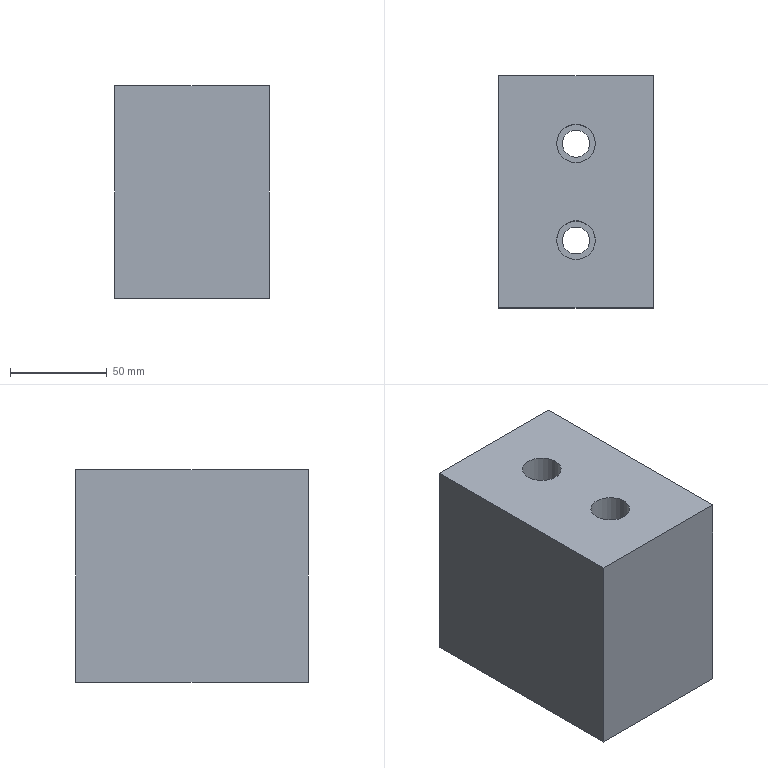Part | NX | features solid 2 | 1 solid | 12 faces | box 80 x 120 x 110 mm | volume 993294 mm3 | plane 8 | cylinder 4 | commonest cylinder face diameters 14 x2 20 x2
STEP:
#1=CARTESIAN_POINT('',(930.,850.,-30.));
#2=VERTEX_POINT('',#1);
#3=CARTESIAN_POINT('',(940.,850.,-30.));
#4=DIRECTION('',(0.,0.,-1.));
#5=DIRECTION('',(-1.,0.,0.));
#6=AXIS2_PLACEMENT_3D('',#3,#4,#5);
#7=CIRCLE('',#6,10.);
#8=EDGE_CURVE('',#2,#2,#7,.T.);
#9=ORIENTED_EDGE('',*,*,#8,.T.);
#10=EDGE_LOOP('',(#9));
#11=FACE_BOUND('',#10,.T.);
#12=CARTESIAN_POINT('',(930.,800.,-30.));
#13=VERTEX_POINT('',#12);
#14=CARTESIAN_POINT('',(940.,800.,-30.));
#15=DIRECTION('',(0.,0.,-1.));
#16=DIRECTION('',(-1.,0.,0.));
#17=AXIS2_PLACEMENT_3D('',#14,#15,#16);
#18=CIRCLE('',#17,10.);
#19=EDGE_CURVE('',#13,#13,#18,.T.);
#20=ORIENTED_EDGE('',*,*,#19,.T.);
#21=EDGE_LOOP('',(#20));
#22=FACE_BOUND('',#21,.T.);
#23=CARTESIAN_POINT('',(980.,765.,-30.));
#24=VERTEX_POINT('',#23);
#25=CARTESIAN_POINT('',(900.,765.,-30.));
#26=VERTEX_POINT('',#25);
#27=CARTESIAN_POINT('',(970.,765.,-30.));
#28=DIRECTION('',(-1.,0.,0.));
#29=VECTOR('',#28,1000.);
#30=LINE('',#27,#29);
#31=EDGE_CURVE('',#24,#26,#30,.T.);
#32=ORIENTED_EDGE('',*,*,#31,.F.);
#33=CARTESIAN_POINT('',(980.,885.,-30.));
#34=VERTEX_POINT('',#33);
#35=CARTESIAN_POINT('',(980.,880.,-30.));
#36=DIRECTION('',(0.,-1.,0.));
#37=VECTOR('',#36,1000.);
#38=LINE('',#35,#37);
#39=EDGE_CURVE('',#34,#24,#38,.T.);
#40=ORIENTED_EDGE('',*,*,#39,.F.);
#41=CARTESIAN_POINT('',(900.,885.,-30.));
#42=VERTEX_POINT('',#41);
#43=CARTESIAN_POINT('',(970.,885.,-30.));
#44=DIRECTION('',(1.,0.,0.));
#45=VECTOR('',#44,1000.);
#46=LINE('',#43,#45);
#47=EDGE_CURVE('',#34,#42,#46,.F.);
#48=ORIENTED_EDGE('',*,*,#47,.T.);
#49=CARTESIAN_POINT('',(900.,880.,-30.));
#50=DIRECTION('',(0.,-1.,0.));
#51=VECTOR('',#50,1000.);
#52=LINE('',#49,#51);
#53=EDGE_CURVE('',#42,#26,#52,.T.);
#54=ORIENTED_EDGE('',*,*,#53,.T.);
#55=EDGE_LOOP('',(#32,#40,#48,#54));
#56=FACE_BOUND('',#55,.T.);
#57=CARTESIAN_POINT('',(970.,880.,-30.));
#58=DIRECTION('',(0.,0.,1.));
#59=DIRECTION('',(0.,-1.,0.));
#60=AXIS2_PLACEMENT_3D('',#57,#58,#59);
#61=PLANE('',#60);
#62=ADVANCED_FACE('',(#11,#22,#56),#61,.T.);
#63=ORIENTED_EDGE('',*,*,#47,.F.);
#64=CARTESIAN_POINT('',(980.,885.,-140.));
#65=VERTEX_POINT('',#64);
#66=CARTESIAN_POINT('',(980.,885.,-30.));
#67=DIRECTION('',(0.,0.,1.));
#68=VECTOR('',#67,1000.);
#69=LINE('',#66,#68);
#70=EDGE_CURVE('',#34,#65,#69,.F.);
#71=ORIENTED_EDGE('',*,*,#70,.T.);
#72=CARTESIAN_POINT('',(900.,885.,-140.));
#73=VERTEX_POINT('',#72);
#74=CARTESIAN_POINT('',(970.,885.,-140.));
#75=DIRECTION('',(-1.,0.,0.));
#76=VECTOR('',#75,1000.);
#77=LINE('',#74,#76);
#78=EDGE_CURVE('',#65,#73,#77,.T.);
#79=ORIENTED_EDGE('',*,*,#78,.T.);
#80=CARTESIAN_POINT('',(900.,885.,-30.));
#81=DIRECTION('',(0.,0.,1.));
#82=VECTOR('',#81,1000.);
#83=LINE('',#80,#82);
#84=EDGE_CURVE('',#42,#73,#83,.F.);
#85=ORIENTED_EDGE('',*,*,#84,.F.);
#86=EDGE_LOOP('',(#63,#71,#79,#85));
#87=FACE_BOUND('',#86,.T.);
#88=CARTESIAN_POINT('',(970.,885.,-30.));
#89=DIRECTION('',(0.,-1.,0.));
#90=DIRECTION('',(0.,0.,-1.));
#91=AXIS2_PLACEMENT_3D('',#88,#89,#90);
#92=PLANE('',#91);
#93=ADVANCED_FACE('',(#87),#92,.F.);
#94=CARTESIAN_POINT('',(947.,850.,-140.));
#95=VERTEX_POINT('',#94);
#96=CARTESIAN_POINT('',(940.,850.,-140.));
#97=DIRECTION('',(0.,0.,1.));
#98=DIRECTION('',(1.,0.,0.));
#99=AXIS2_PLACEMENT_3D('',#96,#97,#98);
#100=CIRCLE('',#99,7.);
#101=EDGE_CURVE('',#95,#95,#100,.F.);
#102=ORIENTED_EDGE('',*,*,#101,.F.);
#103=EDGE_LOOP('',(#102));
#104=FACE_BOUND('',#103,.T.);
#105=CARTESIAN_POINT('',(947.,800.,-140.));
#106=VERTEX_POINT('',#105);
#107=CARTESIAN_POINT('',(940.,800.,-140.));
#108=DIRECTION('',(0.,0.,1.));
#109=DIRECTION('',(1.,0.,0.));
#110=AXIS2_PLACEMENT_3D('',#107,#108,#109);
#111=CIRCLE('',#110,7.);
#112=EDGE_CURVE('',#106,#106,#111,.F.);
#113=ORIENTED_EDGE('',*,*,#112,.F.);
#114=EDGE_LOOP('',(#113));
#115=FACE_BOUND('',#114,.T.);
#116=ORIENTED_EDGE('',*,*,#78,.F.);
#117=CARTESIAN_POINT('',(980.,765.,-140.));
#118=VERTEX_POINT('',#117);
#119=CARTESIAN_POINT('',(980.,880.,-140.));
#120=DIRECTION('',(0.,1.,0.));
#121=VECTOR('',#120,1000.);
#122=LINE('',#119,#121);
#123=EDGE_CURVE('',#65,#118,#122,.F.);
#124=ORIENTED_EDGE('',*,*,#123,.T.);
#125=CARTESIAN_POINT('',(900.,765.,-140.));
#126=VERTEX_POINT('',#125);
#127=CARTESIAN_POINT('',(970.,765.,-140.));
#128=DIRECTION('',(1.,0.,0.));
#129=VECTOR('',#128,1000.);
#130=LINE('',#127,#129);
#131=EDGE_CURVE('',#118,#126,#130,.F.);
#132=ORIENTED_EDGE('',*,*,#131,.T.);
#133=CARTESIAN_POINT('',(900.,880.,-140.));
#134=DIRECTION('',(0.,1.,0.));
#135=VECTOR('',#134,1000.);
#136=LINE('',#133,#135);
#137=EDGE_CURVE('',#73,#126,#136,.F.);
#138=ORIENTED_EDGE('',*,*,#137,.F.);
#139=EDGE_LOOP('',(#116,#124,#132,#138));
#140=FACE_BOUND('',#139,.T.);
#141=CARTESIAN_POINT('',(970.,880.,-140.));
#142=DIRECTION('',(0.,0.,1.));
#143=DIRECTION('',(0.,-1.,0.));
#144=AXIS2_PLACEMENT_3D('',#141,#142,#143);
#145=PLANE('',#144);
#146=ADVANCED_FACE('',(#104,#115,#140),#145,.F.);
#147=ORIENTED_EDGE('',*,*,#137,.T.);
#148=CARTESIAN_POINT('',(900.,765.,-30.));
#149=DIRECTION('',(0.,0.,-1.));
#150=VECTOR('',#149,1000.);
#151=LINE('',#148,#150);
#152=EDGE_CURVE('',#26,#126,#151,.T.);
#153=ORIENTED_EDGE('',*,*,#152,.F.);
#154=ORIENTED_EDGE('',*,*,#53,.F.);
#155=ORIENTED_EDGE('',*,*,#84,.T.);
#156=EDGE_LOOP('',(#147,#153,#154,#155));
#157=FACE_BOUND('',#156,.T.);
#158=CARTESIAN_POINT('',(900.,880.,-30.));
#159=DIRECTION('',(1.,0.,0.));
#160=DIRECTION('',(0.,0.,-1.));
#161=AXIS2_PLACEMENT_3D('',#158,#159,#160);
#162=PLANE('',#161);
#163=ADVANCED_FACE('',(#157),#162,.F.);
#164=CARTESIAN_POINT('',(980.,765.,-30.));
#165=DIRECTION('',(0.,0.,-1.));
#166=VECTOR('',#165,1000.);
#167=LINE('',#164,#166);
#168=EDGE_CURVE('',#24,#118,#167,.T.);
#169=ORIENTED_EDGE('',*,*,#168,.F.);
#170=ORIENTED_EDGE('',*,*,#31,.T.);
#171=ORIENTED_EDGE('',*,*,#152,.T.);
#172=ORIENTED_EDGE('',*,*,#131,.F.);
#173=EDGE_LOOP('',(#169,#170,#171,#172));
#174=FACE_BOUND('',#173,.T.);
#175=CARTESIAN_POINT('',(970.,765.,-30.));
#176=DIRECTION('',(0.,-1.,0.));
#177=DIRECTION('',(0.,0.,-1.));
#178=AXIS2_PLACEMENT_3D('',#175,#176,#177);
#179=PLANE('',#178);
#180=ADVANCED_FACE('',(#174),#179,.T.);
#181=ORIENTED_EDGE('',*,*,#123,.F.);
#182=ORIENTED_EDGE('',*,*,#70,.F.);
#183=ORIENTED_EDGE('',*,*,#39,.T.);
#184=ORIENTED_EDGE('',*,*,#168,.T.);
#185=EDGE_LOOP('',(#181,#182,#183,#184));
#186=FACE_BOUND('',#185,.T.);
#187=CARTESIAN_POINT('',(980.,880.,-30.));
#188=DIRECTION('',(1.,0.,0.));
#189=DIRECTION('',(0.,0.,-1.));
#190=AXIS2_PLACEMENT_3D('',#187,#188,#189);
#191=PLANE('',#190);
#192=ADVANCED_FACE('',(#186),#191,.T.);
#193=ORIENTED_EDGE('',*,*,#112,.T.);
#194=EDGE_LOOP('',(#193));
#195=FACE_BOUND('',#194,.T.);
#196=CARTESIAN_POINT('',(933.,800.,-120.));
#197=VERTEX_POINT('',#196);
#198=CARTESIAN_POINT('',(940.,800.,-120.));
#199=DIRECTION('',(0.,0.,-1.));
#200=DIRECTION('',(-1.,0.,0.));
#201=AXIS2_PLACEMENT_3D('',#198,#199,#200);
#202=CIRCLE('',#201,7.);
#203=EDGE_CURVE('',#197,#197,#202,.T.);
#204=ORIENTED_EDGE('',*,*,#203,.F.);
#205=EDGE_LOOP('',(#204));
#206=FACE_BOUND('',#205,.T.);
#207=CARTESIAN_POINT('',(940.,800.,-230.));
#208=DIRECTION('',(0.,0.,-1.));
#209=DIRECTION('',(-1.,0.,0.));
#210=AXIS2_PLACEMENT_3D('',#207,#208,#209);
#211=CYLINDRICAL_SURFACE('',#210,7.);
#212=ADVANCED_FACE('',(#195,#206),#211,.F.);
#213=ORIENTED_EDGE('',*,*,#203,.T.);
#214=EDGE_LOOP('',(#213));
#215=FACE_BOUND('',#214,.T.);
#216=CARTESIAN_POINT('',(930.,800.,-120.));
#217=VERTEX_POINT('',#216);
#218=CARTESIAN_POINT('',(940.,800.,-120.));
#219=DIRECTION('',(0.,0.,-1.));
#220=DIRECTION('',(-1.,0.,0.));
#221=AXIS2_PLACEMENT_3D('',#218,#219,#220);
#222=CIRCLE('',#221,10.);
#223=EDGE_CURVE('',#217,#217,#222,.T.);
#224=ORIENTED_EDGE('',*,*,#223,.F.);
#225=EDGE_LOOP('',(#224));
#226=FACE_BOUND('',#225,.T.);
#227=CARTESIAN_POINT('',(940.,800.,-120.));
#228=DIRECTION('',(0.,0.,-1.));
#229=DIRECTION('',(-1.,0.,0.));
#230=AXIS2_PLACEMENT_3D('',#227,#228,#229);
#231=PLANE('',#230);
#232=ADVANCED_FACE('',(#215,#226),#231,.F.);
#233=ORIENTED_EDGE('',*,*,#223,.T.);
#234=EDGE_LOOP('',(#233));
#235=FACE_BOUND('',#234,.T.);
#236=ORIENTED_EDGE('',*,*,#19,.F.);
#237=EDGE_LOOP('',(#236));
#238=FACE_BOUND('',#237,.T.);
#239=CARTESIAN_POINT('',(940.,800.,-30.));
#240=DIRECTION('',(0.,0.,-1.));
#241=DIRECTION('',(-1.,0.,0.));
#242=AXIS2_PLACEMENT_3D('',#239,#240,#241);
#243=CYLINDRICAL_SURFACE('',#242,10.);
#244=ADVANCED_FACE('',(#235,#238),#243,.F.);
#245=ORIENTED_EDGE('',*,*,#101,.T.);
#246=EDGE_LOOP('',(#245));
#247=FACE_BOUND('',#246,.T.);
#248=CARTESIAN_POINT('',(933.,850.,-120.));
#249=VERTEX_POINT('',#248);
#250=CARTESIAN_POINT('',(940.,850.,-120.));
#251=DIRECTION('',(0.,0.,-1.));
#252=DIRECTION('',(-1.,0.,0.));
#253=AXIS2_PLACEMENT_3D('',#250,#251,#252);
#254=CIRCLE('',#253,7.);
#255=EDGE_CURVE('',#249,#249,#254,.T.);
#256=ORIENTED_EDGE('',*,*,#255,.F.);
#257=EDGE_LOOP('',(#256));
#258=FACE_BOUND('',#257,.T.);
#259=CARTESIAN_POINT('',(940.,850.,-230.));
#260=DIRECTION('',(0.,0.,-1.));
#261=DIRECTION('',(-1.,0.,0.));
#262=AXIS2_PLACEMENT_3D('',#259,#260,#261);
#263=CYLINDRICAL_SURFACE('',#262,7.);
#264=ADVANCED_FACE('',(#247,#258),#263,.F.);
#265=ORIENTED_EDGE('',*,*,#255,.T.);
#266=EDGE_LOOP('',(#265));
#267=FACE_BOUND('',#266,.T.);
#268=CARTESIAN_POINT('',(930.,850.,-120.));
#269=VERTEX_POINT('',#268);
#270=CARTESIAN_POINT('',(940.,850.,-120.));
#271=DIRECTION('',(0.,0.,-1.));
#272=DIRECTION('',(-1.,0.,0.));
#273=AXIS2_PLACEMENT_3D('',#270,#271,#272);
#274=CIRCLE('',#273,10.);
#275=EDGE_CURVE('',#269,#269,#274,.T.);
#276=ORIENTED_EDGE('',*,*,#275,.F.);
#277=EDGE_LOOP('',(#276));
#278=FACE_BOUND('',#277,.T.);
#279=CARTESIAN_POINT('',(940.,850.,-120.));
#280=DIRECTION('',(0.,0.,-1.));
#281=DIRECTION('',(-1.,0.,0.));
#282=AXIS2_PLACEMENT_3D('',#279,#280,#281);
#283=PLANE('',#282);
#284=ADVANCED_FACE('',(#267,#278),#283,.F.);
#285=ORIENTED_EDGE('',*,*,#275,.T.);
#286=EDGE_LOOP('',(#285));
#287=FACE_BOUND('',#286,.T.);
#288=ORIENTED_EDGE('',*,*,#8,.F.);
#289=EDGE_LOOP('',(#288));
#290=FACE_BOUND('',#289,.T.);
#291=CARTESIAN_POINT('',(940.,850.,-30.));
#292=DIRECTION('',(0.,0.,-1.));
#293=DIRECTION('',(-1.,0.,0.));
#294=AXIS2_PLACEMENT_3D('',#291,#292,#293);
#295=CYLINDRICAL_SURFACE('',#294,10.);
#296=ADVANCED_FACE('',(#287,#290),#295,.F.);
#297=CLOSED_SHELL('',(#62,#93,#146,#163,#180,#192,#212,#232,#244,#264,#284,#296));
#298=MANIFOLD_SOLID_BREP('',#297);
#299=(LENGTH_UNIT()NAMED_UNIT(*)SI_UNIT(.MILLI.,.METRE.));
#300=UNCERTAINTY_MEASURE_WITH_UNIT(LENGTH_MEASURE(0.00001),#299,'','');
#301=(NAMED_UNIT(*)PLANE_ANGLE_UNIT()SI_UNIT($,.RADIAN.));
#302=(NAMED_UNIT(*)SI_UNIT($,.STERADIAN.)SOLID_ANGLE_UNIT());
#303=(GEOMETRIC_REPRESENTATION_CONTEXT(3)GLOBAL_UNCERTAINTY_ASSIGNED_CONTEXT((#300))GLOBAL_UNIT_ASSIGNED_CONTEXT((#299,#301,#302))REPRESENTATION_CONTEXT('',''));
#304=ADVANCED_BREP_SHAPE_REPRESENTATION('',(#298),#303);